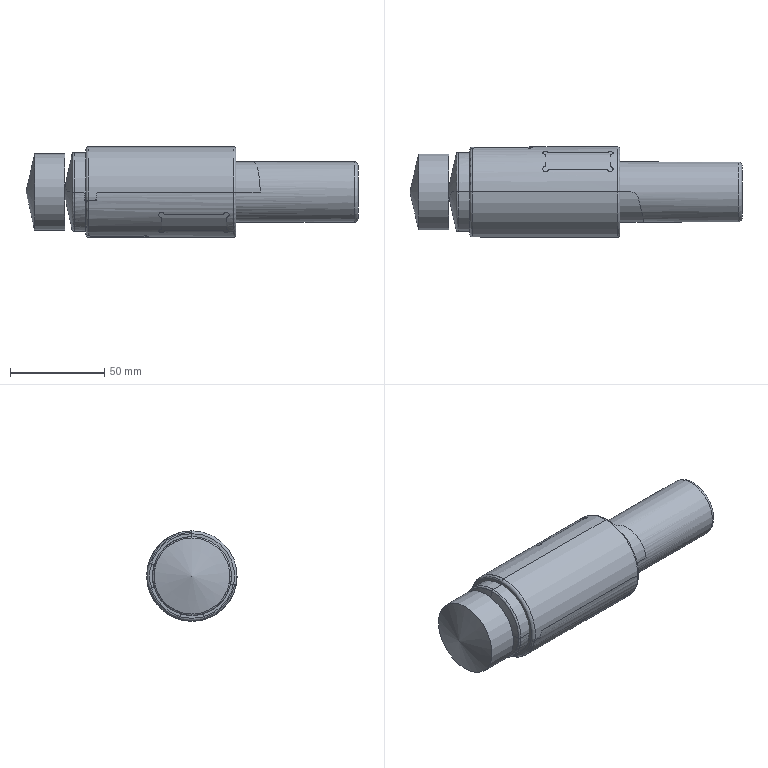NC program | NX | posted with a generic post | part box 176.413 x 48 x 48 mm
Lines 1742 to 2818 of 71815:
(ZLEVEL_PROFILE_COPY , TOOL : D10)
N3482 T10 M6
N3484 G54
N3486 G17 G0 G90 X-59.96 Y-8.562 S3500 M3
N3488 G43 Z33.936 H10
N3490 Z15.781
N3492 G94 G1 X-59.542 Y-8.165 F2000.
N3494 G3 X-59.258 Y-7.206 R1.
N3496 G1 X-59.789 Y-5.
N3498 X-62.069
N3500 G3 X-62.935 Y-5.5 R1.
N3502 G1 X-63.224 Y-6.
N3504 G0 X-59.96 Y-8.563 Z15.562
N3506 G1 X-59.541 Y-8.165
N3508 G3 X-59.258 Y-7.206 R1.
N3510 G1 X-59.789 Y-5.
N3512 X-62.069
N3514 G3 X-62.935 Y-5.5 R1.
N3516 G1 X-63.224 Y-6.
N3518 G0 X-59.96 Y-8.563 Z15.342
N3520 G1 X-59.541 Y-8.166
N3522 G3 X-59.258 Y-7.207 R1.
N3524 G1 X-59.789 Y-5.
N3526 X-62.07
N3528 G3 X-62.936 Y-5.5 R1.
N3530 G1 X-63.224 Y-6.
N3532 G0 X-59.96 Y-8.564 Z15.123
N3534 G1 X-59.541 Y-8.166
N3536 G3 X-59.258 Y-7.207 R1.
N3538 G1 X-59.789 Y-5.
N3540 X-62.07
N3542 G3 X-62.936 Y-5.5 R1.
N3544 G1 X-63.225 Y-6.
N3546 G0 X-59.96 Y-8.565 Z14.904
N3548 G1 X-59.541 Y-8.167
N3550 G3 X-59.257 Y-7.208 R1.
N3552 G1 X-59.789 Y-5.
N3554 X-62.07
N3556 G3 X-62.936 Y-5.5 R1.
N3558 G1 X-63.225 Y-6.
N3560 G0 X-59.959 Y-8.569 Z14.685
N3562 G1 X-59.54 Y-8.171
N3564 G3 X-59.256 Y-7.212 R1.
N3566 G1 X-59.789 Y-5.
N3568 X-62.071
N3570 G3 X-62.937 Y-5.5 R1.
N3572 G1 X-63.225 Y-6.
N3574 G0 X-59.959 Y-8.569 Z14.466
N3576 G1 X-59.54 Y-8.171
N3578 G3 X-59.256 Y-7.212 R1.
N3580 G1 X-59.789 Y-5.
N3582 X-62.071
N3584 G3 X-62.937 Y-5.5 R1.
N3586 G1 X-63.226 Y-6.
N3588 G0 X-59.959 Y-8.569 Z14.247
N3590 G1 X-59.54 Y-8.171
N3592 G3 X-59.256 Y-7.212 R1.
N3594 G1 X-59.789 Y-5.
N3596 X-62.071
N3598 G3 X-62.937 Y-5.5 R1.
N3600 G1 X-63.226 Y-6.
N3602 G0 X-59.959 Y-8.569 Z14.027
N3604 G1 X-59.54 Y-8.171
N3606 G3 X-59.256 Y-7.212 R1.
N3608 G1 X-59.789 Y-5.
N3610 X-62.072
N3612 G3 X-62.938 Y-5.5 R1.
N3614 G1 X-63.226 Y-6.
N3616 G0 X-59.959 Y-8.569 Z13.808
N3618 G1 X-59.54 Y-8.171
N3620 G3 X-59.256 Y-7.212 R1.
N3622 G1 X-59.789 Y-5.
N3624 X-62.072
N3626 G3 X-62.938 Y-5.5 R1.
N3628 G1 X-63.227 Y-6.
N3630 G0 X-59.959 Y-8.569 Z13.589
N3632 G1 X-59.54 Y-8.171
N3634 G3 X-59.256 Y-7.212 R1.
N3636 G1 X-59.789 Y-5.
N3638 X-62.072
N3640 G3 X-62.939 Y-5.5 R1.
N3642 G1 X-63.227 Y-6.
N3644 G0 X-59.959 Y-8.569 Z13.37
N3646 G1 X-59.54 Y-8.171
N3648 G3 X-59.256 Y-7.212 R1.
N3650 G1 X-59.789 Y-5.
N3652 X-62.073
N3654 G3 X-62.939 Y-5.5 R1.
N3656 G1 X-63.228 Y-6.
N3658 G0 X-59.959 Y-8.569 Z13.151
N3660 G1 X-59.54 Y-8.171
N3662 G3 X-59.256 Y-7.212 R1.
N3664 G1 X-59.789 Y-5.
N3666 X-62.073
N3668 G3 X-62.939 Y-5.5 R1.
N3670 G1 X-63.228 Y-6.
N3672 G0 X-59.959 Y-8.569 Z12.932
N3674 G1 X-59.54 Y-8.171
N3676 G3 X-59.256 Y-7.212 R1.
N3678 G1 X-59.789 Y-5.
N3680 X-62.073
N3682 G3 X-62.939 Y-5.5 R1.
N3684 G1 X-63.228 Y-6.
N3686 G0 X-59.959 Y-8.569 Z12.712
N3688 G1 X-59.54 Y-8.171
N3690 G3 X-59.256 Y-7.212 R1.
N3692 G1 X-59.789 Y-5.
N3694 X-62.073
N3696 G3 X-62.939 Y-5.5 R1.
N3698 G1 X-63.228 Y-6.
N3700 G0 X-59.959 Y-8.569 Z12.493
N3702 G1 X-59.54 Y-8.171
N3704 G3 X-59.256 Y-7.212 R1.
N3706 G1 X-59.789 Y-5.
N3708 X-62.073
N3710 G3 X-62.939 Y-5.5 R1.
N3712 G1 X-63.228 Y-6.
N3714 G0 X-59.959 Y-8.569 Z12.274
N3716 G1 X-59.54 Y-8.171
N3718 G3 X-59.256 Y-7.212 R1.
N3720 G1 X-59.789 Y-5.
N3722 X-62.073
N3724 G3 X-62.939 Y-5.5 R1.
N3726 G1 X-63.228 Y-6.
N3728 G0 X-59.959 Y-8.569 Z12.055
N3730 G1 X-59.54 Y-8.171
N3732 G3 X-59.256 Y-7.212 R1.
N3734 G1 X-59.789 Y-5.
N3736 X-62.074
N3738 G3 X-62.94 Y-5.5 R1.
N3740 G1 X-63.228 Y-6.
N3742 G0 X-59.962 Y-8.556 Z11.836
N3744 G1 X-59.543 Y-8.158
N3746 G3 X-59.26 Y-7.199 R1.
N3748 G1 X-59.788 Y-5.001
N3750 X-62.049
N3752 G3 X-62.915 Y-5.501 R1.
N3754 G1 X-63.204 Y-6.001
N3756 G0 X-59.961 Y-8.561 Z11.616
N3758 G1 X-59.542 Y-8.163
N3760 G3 X-59.258 Y-7.204 R1.
N3762 G1 X-59.787 Y-5.006
N3764 X-62.048
N3766 G3 X-62.914 Y-5.506 R1.
N3768 G1 X-63.203 Y-6.006
N3770 G0 X-59.958 Y-8.57 Z11.397
N3772 G1 X-59.54 Y-8.172
N3774 G3 X-59.256 Y-7.213 R1.
N3776 G1 X-59.785 Y-5.015
N3778 X-62.046
N3780 G3 X-62.912 Y-5.515 R1.
N3782 G1 X-63.201 Y-6.015
N3784 G0 X-59.955 Y-8.583 Z11.178
N3786 G1 X-59.537 Y-8.185
N3788 G3 X-59.253 Y-7.226 R1.
N3790 G1 X-59.782 Y-5.028
N3792 X-62.043
N3794 G3 X-62.909 Y-5.528 R1.
N3796 G1 X-63.197 Y-6.028
N3798 G0 X-59.951 Y-8.6 Z10.959
N3800 G1 X-59.532 Y-8.202
N3802 G3 X-59.249 Y-7.244 R1.
N3804 G1 X-59.778 Y-5.045
N3806 X-62.039
N3808 G3 X-62.905 Y-5.545 R1.
N3810 G1 X-63.193 Y-6.045
N3812 G0 X-59.946 Y-8.621 Z10.74
N3814 G1 X-59.527 Y-8.224
N3816 G3 X-59.244 Y-7.265 R1.
N3818 G1 X-59.773 Y-5.066
N3820 X-62.034
N3822 G3 X-62.9 Y-5.566 R1.
N3824 G1 X-63.188 Y-6.066
N3826 G0 X-59.94 Y-8.646 Z10.521
N3828 G1 X-59.521 Y-8.249
N3830 G3 X-59.238 Y-7.29 R1.
N3832 G1 X-59.767 Y-5.092
N3834 X-62.027
N3836 G3 X-62.894 Y-5.592 R1.
N3838 G1 X-63.182 Y-6.092
N3840 G0 X-59.933 Y-8.676 Z10.301
N3842 G1 X-59.514 Y-8.278
N3844 G3 X-59.231 Y-7.319 R1.
N3846 G1 X-59.759 Y-5.121
N3848 X-62.02
N3850 G3 X-62.886 Y-5.621 R1.
N3852 G1 X-63.175 Y-6.121
N3854 G0 X-59.925 Y-8.709 Z10.082
N3856 G1 X-59.506 Y-8.311
N3858 G3 X-59.223 Y-7.352 R1.
N3860 G1 X-59.751 Y-5.154
N3862 X-62.012
N3864 G3 X-62.878 Y-5.654 R1.
N3866 G1 X-63.167 Y-6.154
N3868 G0 X-59.916 Y-8.747 Z9.863
N3870 G1 X-59.497 Y-8.349
N3872 G3 X-59.214 Y-7.39 R1.
N3874 G1 X-59.742 Y-5.192
N3876 X-62.003
N3878 G3 X-62.869 Y-5.692 R1.
N3880 G1 X-63.158 Y-6.192
N3882 G0 X-59.906 Y-8.788 Z9.644
N3884 G1 X-59.487 Y-8.391
N3886 G3 X-59.204 Y-7.432 R1.
N3888 G1 X-59.732 Y-5.234
N3890 X-61.993
N3892 G3 X-62.859 Y-5.734 R1.
N3894 G1 X-63.148 Y-6.234
N3896 G0 X-59.895 Y-8.834 Z9.425
N3898 G1 X-59.476 Y-8.437
N3900 G3 X-59.193 Y-7.478 R1.
N3902 G1 X-59.721 Y-5.28
N3904 X-61.982
N3906 G3 X-62.848 Y-5.78 R1.
N3908 G1 X-63.137 Y-6.28
N3910 G0 X-59.883 Y-8.885 Z9.205
N3912 G1 X-59.464 Y-8.487
N3914 G3 X-59.18 Y-7.528 R1.
N3916 G1 X-59.709 Y-5.33
N3918 X-61.97
N3920 G3 X-62.836 Y-5.83 R1.
N3922 G1 X-63.125 Y-6.33
N3924 G0 X-59.869 Y-8.939 Z8.986
N3926 G1 X-59.451 Y-8.542
N3928 G3 X-59.167 Y-7.583 R1.
N3930 G1 X-59.696 Y-5.385
N3932 X-61.957
N3934 G3 X-62.823 Y-5.885 R1.
N3936 G1 X-63.112 Y-6.385
N3938 G0 X-59.855 Y-8.998 Z8.767
N3940 G1 X-59.437 Y-8.601
N3942 G3 X-59.153 Y-7.642 R1.
N3944 G1 X-59.682 Y-5.444
N3946 X-61.943
N3948 G3 X-62.809 Y-5.944 R1.
N3950 G1 X-63.097 Y-6.444
N3952 G0 X-59.84 Y-9.062 Z8.548
N3954 G1 X-59.421 Y-8.664
N3956 G3 X-59.138 Y-7.706 R1.
N3958 G1 X-59.667 Y-5.507
N3960 X-61.927
N3962 G3 X-62.794 Y-6.007 R1.
N3964 G1 X-63.082 Y-6.507
N3966 G0 X-59.824 Y-9.13 Z8.329
N3968 G1 X-59.405 Y-8.733
N3970 G3 X-59.121 Y-7.774 R1.
N3972 G1 X-59.65 Y-5.575
N3974 X-61.911
N3976 G3 X-62.777 Y-6.075 R1.
N3978 G1 X-63.066 Y-6.575
N3980 G0 X-59.806 Y-9.203 Z8.11
N3982 G1 X-59.387 Y-8.805
N3984 G3 X-59.104 Y-7.846 R1.
N3986 G1 X-59.633 Y-5.648
N3988 X-61.894
N3990 G3 X-62.76 Y-6.148 R1.
N3992 G1 X-63.048 Y-6.648
N3994 G0 X-59.787 Y-9.28 Z7.89
N3996 G1 X-59.369 Y-8.883
N3998 G3 X-59.085 Y-7.924 R1.
N4000 G1 X-59.614 Y-5.726
N4002 X-61.875
N4004 G3 X-62.741 Y-6.226 R1.
N4006 G1 X-63.03 Y-6.726
N4008 G0 X-59.768 Y-9.363 Z7.671
N4010 G1 X-59.349 Y-8.965
N4012 G3 X-59.065 Y-8.006 R1.
N4014 G1 X-59.594 Y-5.808
N4016 X-61.855
N4018 G3 X-62.721 Y-6.308 R1.
N4020 G1 X-63.01 Y-6.808
N4022 G0 X-59.747 Y-9.45 Z7.452
N4024 G1 X-59.328 Y-9.052
N4026 G3 X-59.044 Y-8.093 R1.
N4028 G1 X-59.573 Y-5.895
N4030 X-61.834
N4032 G3 X-62.7 Y-6.395 R1.
N4034 G1 X-62.989 Y-6.895
N4036 G0 X-59.724 Y-9.542 Z7.233
N4038 G1 X-59.306 Y-9.145
N4040 G3 X-59.022 Y-8.186 R1.
N4042 G1 X-59.551 Y-5.988
N4044 X-61.812
N4046 G3 X-62.678 Y-6.488 R1.
N4048 G1 X-62.967 Y-6.988
N4050 G0 X-59.701 Y-9.64 Z7.014
N4052 G1 X-59.282 Y-9.242
N4054 G3 X-58.999 Y-8.283 R1.
N4056 G1 X-59.528 Y-6.085
N4058 X-61.789
N4060 G3 X-62.655 Y-6.585 R1.
N4062 G1 X-62.943 Y-7.085
N4064 G0 X-59.676 Y-9.743 Z6.795
N4066 G1 X-59.258 Y-9.345
N4068 G3 X-58.974 Y-8.386 R1.
N4070 G1 X-59.503 Y-6.188
N4072 X-61.764
N4074 G3 X-62.63 Y-6.688 R1.
N4076 G1 X-62.918 Y-7.188
N4078 G0 X-59.65 Y-9.851 Z6.575
N4080 G1 X-59.232 Y-9.453
N4082 G3 X-58.948 Y-8.494 R1.
N4084 G1 X-59.477 Y-6.296
N4086 X-61.738
N4088 G3 X-62.604 Y-6.796 R1.
N4090 G1 X-62.892 Y-7.296
N4092 G0 X-59.623 Y-9.965 Z6.356
N4094 G1 X-59.204 Y-9.567
N4096 G3 X-58.921 Y-8.608 R1.
N4098 G1 X-59.449 Y-6.41
N4100 X-61.71
N4102 G3 X-62.576 Y-6.91 R1.
N4104 G1 X-62.865 Y-7.41
N4106 G0 X-59.594 Y-10.085 Z6.137
N4108 G1 X-59.175 Y-9.687
N4110 G3 X-58.892 Y-8.728 R1.
N4112 G1 X-59.421 Y-6.53
N4114 X-61.682
N4116 G3 X-62.548 Y-7.03 R1.
N4118 G1 X-62.836 Y-7.53
N4120 G0 X-59.564 Y-10.21 Z5.918
N4122 G1 X-59.145 Y-9.813
N4124 G3 X-58.862 Y-8.854 R1.
N4126 G1 X-59.39 Y-6.656
N4128 X-61.651
N4130 G3 X-62.517 Y-7.156 R1.
N4132 G1 X-62.806 Y-7.656
N4134 G0 X-59.532 Y-10.342 Z5.699
N4136 G1 X-59.113 Y-9.945
N4138 G3 X-58.83 Y-8.986 R1.
N4140 G1 X-59.359 Y-6.788
N4142 X-61.62
N4144 G3 X-62.486 Y-7.288 R1.
N4146 G1 X-62.774 Y-7.788
N4148 G0 X-59.499 Y-10.481 Z5.479
N4150 G1 X-59.08 Y-10.083
N4152 G3 X-58.796 Y-9.124 R1.
N4154 G1 X-59.325 Y-6.926
N4156 X-61.586
N4158 G3 X-62.452 Y-7.426 R1.
N4160 G1 X-62.741 Y-7.926
N4162 G0 X-59.464 Y-10.626 Z5.26
N4164 G1 X-59.045 Y-10.229
N4166 G3 X-58.762 Y-9.27 R1.
N4168 G1 X-59.29 Y-7.071
N4170 X-61.551
N4172 G3 X-62.417 Y-7.571 R1.
N4174 G1 X-62.706 Y-8.071
N4176 G0 X-59.427 Y-10.779 Z5.041
N4178 G1 X-59.008 Y-10.381
N4180 G3 X-58.725 Y-9.422 R1.
N4182 G1 X-59.254 Y-7.224
N4184 X-61.515
N4186 G3 X-62.381 Y-7.724 R1.
N4188 G1 X-62.669 Y-8.224
N4190 G0 X-59.389 Y-10.938 Z4.822
N4192 G1 X-58.97 Y-10.541
N4194 G3 X-58.686 Y-9.582 R1.
N4196 G1 X-59.215 Y-7.384
N4198 X-61.476
N4200 G3 X-62.342 Y-7.884 R1.
N4202 G1 X-62.631 Y-8.384
N4204 G0 X-59.348 Y-11.106 Z4.603
N4206 G1 X-58.93 Y-10.708
N4208 G3 X-58.646 Y-9.749 R1.
N4210 G1 X-59.175 Y-7.551
N4212 X-61.436
N4214 G3 X-62.302 Y-8.051 R1.
N4216 G1 X-62.591 Y-8.551
N4218 G0 X-59.306 Y-11.282 Z4.384
N4220 G1 X-58.887 Y-10.884
N4222 G3 X-58.604 Y-9.925 R1.
N4224 G1 X-59.133 Y-7.727
N4226 X-61.394
N4228 G3 X-62.26 Y-8.227 R1.
N4230 G1 X-62.548 Y-8.727
N4232 G0 X-59.262 Y-11.466 Z4.164
N4234 G1 X-58.843 Y-11.069
N4236 G3 X-58.559 Y-10.11 R1.
N4238 G1 X-59.088 Y-7.911
N4240 X-61.349
N4242 G3 X-62.215 Y-8.411 R1.
N4244 G1 X-62.504 Y-8.911
N4246 G0 X-59.215 Y-11.66 Z3.945
N4248 G1 X-58.796 Y-11.262
N4250 G3 X-58.513 Y-10.303 R1.
N4252 G1 X-59.042 Y-8.105
N4254 X-61.303
N4256 G3 X-62.169 Y-8.605 R1.
N4258 G1 X-62.457 Y-9.105
N4260 G0 X-59.166 Y-11.863 Z3.726
N4262 G1 X-58.748 Y-11.466
N4264 G3 X-58.464 Y-10.507 R1.
N4266 G1 X-58.993 Y-8.309
N4268 X-61.254
N4270 G3 X-62.12 Y-8.809 R1.
N4272 G1 X-62.408 Y-9.309
N4274 G0 X-59.115 Y-12.077 Z3.507
N4276 G1 X-58.696 Y-11.68
N4278 G3 X-58.412 Y-10.721 R1.
N4280 G1 X-58.941 Y-8.523
N4282 X-61.202
N4284 G3 X-62.068 Y-9.023 R1.
N4286 G1 X-62.357 Y-9.523
N4288 G0 X-59.06 Y-12.303 Z3.288
N4290 G1 X-58.642 Y-11.905
N4292 G3 X-58.358 Y-10.946 R1.
N4294 G1 X-58.887 Y-8.748
N4296 X-61.148
N4298 G3 X-62.014 Y-9.248 R1.
N4300 G1 X-62.303 Y-9.748
N4302 G0 X-59.003 Y-12.541 Z3.068
N4304 G1 X-58.585 Y-12.143
N4306 G3 X-58.301 Y-11.184 R1.
N4308 G1 X-58.83 Y-8.986
N4310 X-61.091
N4312 G3 X-61.957 Y-9.486 R1.
N4314 G1 X-62.245 Y-9.986
N4316 G0 X-58.943 Y-12.792 Z2.849
N4318 G1 X-58.524 Y-12.394
N4320 G3 X-58.241 Y-11.435 R1.
N4322 G1 X-58.769 Y-9.237
N4324 X-61.03
N4326 G3 X-61.896 Y-9.737 R1.
N4328 G1 X-62.185 Y-10.237
N4330 G0 X-58.879 Y-13.058 Z2.63
N4332 G1 X-58.46 Y-12.66
N4334 G3 X-58.177 Y-11.701 R1.
N4336 G1 X-58.705 Y-9.503
N4338 X-60.966
N4340 G3 X-61.832 Y-10.003 R1.
N4342 G1 X-62.121 Y-10.503
N4344 G0 X-58.811 Y-13.34 Z2.411
N4346 G1 X-58.392 Y-12.943
N4348 G3 X-58.109 Y-11.984 R1.
N4350 G1 X-58.637 Y-9.785
N4352 X-60.898
N4354 G3 X-61.764 Y-10.285 R1.
N4356 G1 X-62.053 Y-10.785
N4358 G0 X-58.739 Y-13.641 Z2.192
N4360 G1 X-58.32 Y-13.244
N4362 G3 X-58.036 Y-12.285 R1.
N4364 G1 X-58.565 Y-10.086
N4366 X-60.826
N4368 G3 X-61.692 Y-10.586 R1.
N4370 G1 X-61.981 Y-11.086
N4372 G0 X-58.661 Y-13.963 Z1.973
N4374 G1 X-58.242 Y-13.565
N4376 G3 X-57.959 Y-12.606 R1.
N4378 G1 X-58.488 Y-10.408
N4380 X-60.749
N4382 G3 X-61.615 Y-10.908 R1.
N4384 G1 X-61.903 Y-11.408
N4386 G0 X-58.578 Y-14.309 Z1.753
N4388 G1 X-58.159 Y-13.912
N4390 G3 X-57.876 Y-12.953 R1.
N4392 G1 X-58.404 Y-10.754
N4394 X-60.665
N4396 G3 X-61.531 Y-11.254 R1.
N4398 G1 X-61.82 Y-11.754
N4400 G0 X-58.488 Y-14.684 Z1.534
N4402 G1 X-58.069 Y-14.286
N4404 G3 X-57.786 Y-13.327 R1.
N4406 G1 X-58.314 Y-11.129
N4408 X-60.575
N4410 G3 X-61.441 Y-11.629 R1.
N4412 G1 X-61.73 Y-12.129
N4414 G0 X-58.389 Y-15.093 Z1.315
N4416 G1 X-57.971 Y-14.695
N4418 G3 X-57.687 Y-13.736 R1.
N4420 G1 X-58.216 Y-11.538
N4422 X-60.477
N4424 G3 X-61.343 Y-12.038 R1.
N4426 G1 X-61.632 Y-12.538
N4428 G0 X-58.281 Y-15.545 Z1.096
N4430 G1 X-57.862 Y-15.147
N4432 G3 X-57.578 Y-14.188 R1.
N4434 G1 X-58.107 Y-11.99
N4436 X-60.368
N4438 G3 X-61.234 Y-12.49 R1.
N4440 G1 X-61.523 Y-12.99
N4442 G0 X-58.159 Y-16.052 Z0.877
N4444 G1 X-57.74 Y-15.655
N4446 G3 X-57.456 Y-14.696 R1.
N4448 G1 X-57.985 Y-12.498
N4450 X-60.246
N4452 G3 X-61.112 Y-12.998 R1.
N4454 G1 X-61.401 Y-13.498
N4456 G0 X-58.018 Y-16.637 Z0.658
N4458 G1 X-57.599 Y-16.239
N4460 G3 X-57.316 Y-15.281 R1.
N4462 G1 X-57.844 Y-13.082
N4464 X-60.105
N4466 G3 X-60.971 Y-13.582 R1.
N4468 G1 X-61.26 Y-14.082
N4470 G0 X-57.842 Y-17.368 Z0.438
N4472 G1 X-57.424 Y-16.97
N4474 G3 X-57.14 Y-16.011 R1.
N4476 G1 X-57.675 Y-13.786
N4478 X-59.942
N4480 G3 X-60.808 Y-14.286 R1.
N4482 G1 X-61.097 Y-14.786
N4484 G0 X-57.613 Y-18.321 Z0.219
N4486 G1 X-57.194 Y-17.923
N4488 G3 X-56.911 Y-16.964 R1.
N4490 G1 X-57.451 Y-14.717
N4492 X-59.723
N4494 G3 X-60.589 Y-15.217 R1.
N4496 G1 X-60.877 Y-15.717
N4498 G0 X-57.177 Y-20.13 Z0.
N4500 G1 X-56.758 Y-19.732
N4502 G3 X-56.475 Y-18.773 R1.
N4504 G1 X-56.814 Y-17.369
N4506 X-56.861 Y-17.169
N4508 X-57.007 Y-16.563
N4510 X-59.331
N4512 G3 X-60.197 Y-17.064 R1.
N4514 G1 X-60.486 Y-17.564
N4516 G0 Z30.274
(ZLEVEL_PROFILE_COPY_COPY , TOOL : D10)
N4518 X-80.529 Y25.398 S2500
N4520 Z24.082
N4522 Y18.689 Z17.374
N4524 G1 X-99.3 Y17.993 Z16.678 F1000.
N4526 Y16.609 Z17.924
N4528 X-87.2 Y16.161 Z17.476
N4530 X-75.1 F2000.
N4532 Y17.476 Z16.161
N4534 X-99.3
N4536 Y16.161 Z17.476
N4538 X-87.2
N4540 X-75.15 Y16.012 Z17.327
N4542 X-75.1 Y16.043 Z17.293
N4544 Y16.177 Z17.154
N4546 Y17.323 Z16.008
N4548 X-99.3
N4550 Y16.008 Z17.323
N4552 X-87.2
N4554 X-75.15 Y15.86 Z17.175
N4556 X-75.1 Y15.891 Z17.141
N4558 Y16.025 Z17.002
N4560 Y17.171 Z15.856
N4562 X-99.3
N4564 Y15.856 Z17.171
N4566 X-87.2
N4568 X-75.15 Y15.707 Z17.022
N4570 X-75.1 Y15.739 Z16.989
N4572 Y15.873 Z16.85
N4574 Y17.019 Z15.704
N4576 X-99.3
N4578 Y15.704 Z17.019
N4580 X-87.2
N4582 X-75.15 Y15.555 Z16.87
N4584 X-75.1 Y15.586 Z16.836
N4586 Y15.72 Z16.698
N4588 Y16.867 Z15.551
N4590 X-99.3
N4592 Y15.551 Z16.867
N4594 X-87.2
N4596 X-75.15 Y15.403 Z16.718
N4598 X-75.1 Y15.434 Z16.684
N4600 Y15.568 Z16.545
N4602 Y16.714 Z15.399
N4604 X-99.3
N4606 Y15.399 Z16.714
N4608 X-87.2
N4610 X-75.15 Y15.25 Z16.566
N4612 X-75.1 Y15.282 Z16.532
N4614 Y15.416 Z16.393
N4616 Y16.562 Z15.247
N4618 X-99.3
N4620 Y15.247 Z16.562
N4622 X-87.2
N4624 X-75.15 Y15.098 Z16.413
N4626 X-75.1 Y15.13 Z16.379
N4628 Y15.263 Z16.241
N4630 Y16.41 Z15.094
N4632 X-99.3
N4634 Y15.094 Z16.41
N4636 X-87.2
N4638 X-75.15 Y14.946 Z16.261
N4640 X-75.1 Y14.977 Z16.227
N4642 Y15.111 Z16.088
N4644 Y16.257 Z14.942
N4646 X-99.3
N4648 Y14.942 Z16.257
N4650 X-87.2
N4652 X-75.15 Y14.793 Z16.109
N4654 X-75.1 Y14.825 Z16.075
N4656 Y14.959 Z15.936
N4658 Y16.105 Z14.79
N4660 X-99.3
N4662 Y14.79 Z16.105
N4664 X-87.2
N4666 X-75.15 Y14.641 Z15.956
N4668 X-75.1 Y14.673 Z15.923
N4670 Y14.807 Z15.784
N4672 Y15.953 Z14.638
N4674 X-99.3
N4676 Y14.638 Z15.953
N4678 X-87.2
N4680 X-75.15 Y14.489 Z15.804
N4682 X-75.1 Y14.52 Z15.77
N4684 Y14.654 Z15.631
N4686 Y15.801 Z14.485
N4688 X-99.3
N4690 Y14.485 Z15.801
N4692 X-87.2
N4694 X-75.15 Y14.337 Z15.652
N4696 X-75.1 Y14.368 Z15.618
N4698 Y14.502 Z15.479
N4700 Y15.648 Z14.333
N4702 X-99.3
N4704 Y14.333 Z15.648
N4706 X-87.2
N4708 X-75.15 Y14.184 Z15.499
N4710 X-75.1 Y14.216 Z15.466
N4712 Y14.35 Z15.327
N4714 Y15.496 Z14.181
N4716 X-99.3
N4718 Y14.181 Z15.496
N4720 X-87.2
N4722 X-75.15 Y14.032 Z15.347
N4724 X-75.1 Y14.063 Z15.313
N4726 Y14.197 Z15.175
N4728 Y15.344 Z14.028
N4730 X-99.3
N4732 Y14.028 Z15.344
N4734 X-87.2
N4736 X-75.15 Y13.88 Z15.195
N4738 X-75.1 Y13.911 Z15.161
N4740 Y14.045 Z15.022
N4742 Y15.191 Z13.876
N4744 X-99.3
N4746 Y13.876 Z15.191
N4748 X-87.2
N4750 X-75.15 Y13.727 Z15.043
N4752 X-75.1 Y13.759 Z15.009
N4754 Y13.893 Z14.87
N4756 Y15.039 Z13.724
N4758 X-99.3
N4760 Y13.724 Z15.039
N4762 X-87.2
N4764 X-75.15 Y13.575 Z14.89
N4766 X-75.1 Y13.607 Z14.856
N4768 Y13.741 Z14.718
N4770 Y14.887 Z13.572
N4772 X-99.3
N4774 Y13.572 Z14.887
N4776 X-87.2
N4778 X-75.15 Y13.423 Z14.738
N4780 X-75.1 Y13.454 Z14.704
N4782 Y13.588 Z14.565
N4784 Y14.734 Z13.419
N4786 X-99.3
N4788 Y13.419 Z14.734
N4790 X-87.2
N4792 X-75.15 Y13.27 Z14.586
N4794 X-75.1 Y13.302 Z14.552
N4796 Y13.436 Z14.413
N4798 Y14.582 Z13.267
N4800 X-99.3
N4802 Y13.267 Z14.582
N4804 X-87.2
N4806 X-75.15 Y13.118 Z14.433
N4808 X-75.1 Y13.15 Z14.4
N4810 Y13.284 Z14.261
N4812 Y14.43 Z13.115
N4814 X-99.3
N4816 Y13.115 Z14.43
N4818 X-87.2
N4820 X-75.15 Y12.966 Z14.281
N4822 X-75.1 Y12.997 Z14.247
N4824 Y13.131 Z14.109
N4826 Y14.278 Z12.962
N4828 X-99.3
N4830 Y12.962 Z14.278
N4832 X-87.2
N4834 X-75.15 Y12.814 Z14.129
N4836 X-75.1 Y12.845 Z14.095
N4838 Y12.979 Z13.956
N4840 Y14.125 Z12.81
N4842 X-99.3
N4844 Y12.81 Z14.125
N4846 X-87.2
N4848 X-75.15 Y12.661 Z13.977
N4850 X-75.1 Y12.693 Z13.943
N4852 Y12.827 Z13.804
N4854 Y13.973 Z12.658
N4856 X-99.3
N4858 Y12.658 Z13.973
N4860 X-87.2
N4862 X-75.15 Y12.509 Z13.824
N4864 X-75.1 Y12.541 Z13.79
N4866 Y12.674 Z13.652
N4868 Y13.821 Z12.505
N4870 X-99.3
N4872 Y12.505 Z13.821
N4874 X-75.1
N4876 Y12.674 Z13.652
N4878 Y13.735 Z14.712
N4880 G0 Y24.255 Z25.233
(ZLEVEL_PROFILE_COPY_COPY_COPY_1 , TOOL : D10)
N4882 X-80.529 Y-25.398
N4884 Z-24.082
N4886 Y-18.689 Z-17.374
N4888 G1 X-99.3 Y-17.993 Z-16.678 F1000.
N4890 Y-16.609 Z-17.924
N4892 X-87.2 Y-16.161 Z-17.476
N4894 X-75.1 F2000.
N4896 Y-17.476 Z-16.161
N4898 X-99.3
N4900 Y-16.161 Z-17.476
N4902 X-87.2
N4904 X-75.15 Y-16.012 Z-17.327
N4906 X-75.1 Y-16.043 Z-17.293
N4908 Y-16.177 Z-17.154
N4910 Y-17.323 Z-16.008
N4912 X-99.3
N4914 Y-16.008 Z-17.323
N4916 X-87.2
N4918 X-75.15 Y-15.86 Z-17.175
N4920 X-75.1 Y-15.891 Z-17.141
N4922 Y-16.025 Z-17.002
N4924 Y-17.171 Z-15.856
N4926 X-99.3
N4928 Y-15.856 Z-17.171
N4930 X-87.2
N4932 X-75.15 Y-15.707 Z-17.022
N4934 X-75.1 Y-15.739 Z-16.989
N4936 Y-15.873 Z-16.85
N4938 Y-17.019 Z-15.704
N4940 X-99.3
N4942 Y-15.704 Z-17.019
N4944 X-87.2
N4946 X-75.15 Y-15.555 Z-16.87
N4948 X-75.1 Y-15.586 Z-16.836
N4950 Y-15.72 Z-16.698
N4952 Y-16.867 Z-15.551
N4954 X-99.3
N4956 Y-15.551 Z-16.867
N4958 X-87.2
N4960 X-75.15 Y-15.403 Z-16.718
N4962 X-75.1 Y-15.434 Z-16.684
N4964 Y-15.568 Z-16.545
N4966 Y-16.714 Z-15.399
N4968 X-99.3
N4970 Y-15.399 Z-16.714
N4972 X-87.2
N4974 X-75.15 Y-15.25 Z-16.566
N4976 X-75.1 Y-15.282 Z-16.532
N4978 Y-15.416 Z-16.393
N4980 Y-16.562 Z-15.247
N4982 X-99.3
N4984 Y-15.247 Z-16.562
N4986 X-87.2
N4988 X-75.15 Y-15.098 Z-16.413
N4990 X-75.1 Y-15.13 Z-16.379
N4992 Y-15.263 Z-16.241
N4994 Y-16.41 Z-15.094
N4996 X-99.3
N4998 Y-15.094 Z-16.41
N5000 X-87.2
N5002 X-75.15 Y-14.946 Z-16.261
N5004 X-75.1 Y-14.977 Z-16.227
N5006 Y-15.111 Z-16.088
N5008 Y-16.257 Z-14.942
N5010 X-99.3
N5012 Y-14.942 Z-16.257
N5014 X-87.2
N5016 X-75.15 Y-14.793 Z-16.109
N5018 X-75.1 Y-14.825 Z-16.075
N5020 Y-14.959 Z-15.936
N5022 Y-16.105 Z-14.79
N5024 X-99.3
N5026 Y-14.79 Z-16.105
N5028 X-87.2
N5030 X-75.15 Y-14.641 Z-15.956
N5032 X-75.1 Y-14.673 Z-15.923
N5034 Y-14.807 Z-15.784
N5036 Y-15.953 Z-14.638
N5038 X-99.3
N5040 Y-14.638 Z-15.953
N5042 X-87.2
N5044 X-75.15 Y-14.489 Z-15.804
N5046 X-75.1 Y-14.52 Z-15.77
N5048 Y-14.654 Z-15.631
N5050 Y-15.801 Z-14.485
N5052 X-99.3
N5054 Y-14.485 Z-15.801
N5056 X-87.2
N5058 X-75.15 Y-14.337 Z-15.652
N5060 X-75.1 Y-14.368 Z-15.618
N5062 Y-14.502 Z-15.479
N5064 Y-15.648 Z-14.333
N5066 X-99.3
N5068 Y-14.333 Z-15.648
N5070 X-87.2
N5072 X-75.15 Y-14.184 Z-15.499
N5074 X-75.1 Y-14.216 Z-15.466
N5076 Y-14.35 Z-15.327
N5078 Y-15.496 Z-14.181
N5080 X-99.3
N5082 Y-14.181 Z-15.496
N5084 X-87.2
N5086 X-75.15 Y-14.032 Z-15.347
N5088 X-75.1 Y-14.063 Z-15.313
N5090 Y-14.197 Z-15.175
N5092 Y-15.344 Z-14.028
N5094 X-99.3
N5096 Y-14.028 Z-15.344
N5098 X-87.2
N5100 X-75.15 Y-13.88 Z-15.195
N5102 X-75.1 Y-13.911 Z-15.161
N5104 Y-14.045 Z-15.022
N5106 Y-15.191 Z-13.876
N5108 X-99.3
N5110 Y-13.876 Z-15.191
N5112 X-87.2
N5114 X-75.15 Y-13.727 Z-15.043
N5116 X-75.1 Y-13.759 Z-15.009
N5118 Y-13.893 Z-14.87
N5120 Y-15.039 Z-13.724
N5122 X-99.3
N5124 Y-13.724 Z-15.039
N5126 X-87.2
N5128 X-75.15 Y-13.575 Z-14.89
N5130 X-75.1 Y-13.607 Z-14.856
N5132 Y-13.741 Z-14.718
N5134 Y-14.887 Z-13.572
N5136 X-99.3
N5138 Y-13.572 Z-14.887
N5140 X-87.2
N5142 X-75.15 Y-13.423 Z-14.738
N5144 X-75.1 Y-13.454 Z-14.704
N5146 Y-13.588 Z-14.565
N5148 Y-14.734 Z-13.419
N5150 X-99.3
N5152 Y-13.419 Z-14.734
N5154 X-87.2
N5156 X-75.15 Y-13.27 Z-14.586
N5158 X-75.1 Y-13.302 Z-14.552
N5160 Y-13.436 Z-14.413
N5162 Y-14.582 Z-13.267
N5164 X-99.3
N5166 Y-13.267 Z-14.582
N5168 X-87.2
N5170 X-75.15 Y-13.118 Z-14.433
N5172 X-75.1 Y-13.15 Z-14.4
N5174 Y-13.284 Z-14.261
N5176 Y-14.43 Z-13.115
N5178 X-99.3
N5180 Y-13.115 Z-14.43
N5182 X-87.2
N5184 X-75.15 Y-12.966 Z-14.281
N5186 X-75.1 Y-12.997 Z-14.247
N5188 Y-13.131 Z-14.109
N5190 Y-14.278 Z-12.962
N5192 X-99.3
N5194 Y-12.962 Z-14.278
N5196 X-87.2
N5198 X-75.15 Y-12.814 Z-14.129
N5200 X-75.1 Y-12.845 Z-14.095
N5202 Y-12.979 Z-13.956
N5204 Y-14.125 Z-12.81
N5206 X-99.3
N5208 Y-12.81 Z-14.125
N5210 X-87.2
N5212 X-75.15 Y-12.661 Z-13.977
N5214 X-75.1 Y-12.693 Z-13.943
N5216 Y-12.827 Z-13.804
N5218 Y-13.973 Z-12.658
N5220 X-99.3
N5222 Y-12.658 Z-13.973
N5224 X-87.2
N5226 X-75.15 Y-12.509 Z-13.824
N5228 X-75.1 Y-12.541 Z-13.79
N5230 Y-12.674 Z-13.652
N5232 Y-13.821 Z-12.505
N5234 X-99.3
N5236 Y-12.505 Z-13.821
N5238 X-75.1
N5240 Y-12.674 Z-13.652
N5242 Y-13.735 Z-14.712
N5244 G0 Y-24.255 Z-25.233
(ZLEVEL_PROFILE_COPY_COPY_COPY_2 , TOOL : D10)
N5246 X-80.529 Y24.082
N5248 Z-25.398
N5250 Y17.374 Z-18.689
N5252 G1 X-99.3 Y16.678 Z-17.993 F1000.
N5254 Y17.924 Z-16.609
N5256 X-87.2 Y17.476 Z-16.161
N5258 X-75.1 F2000.
N5260 Y16.161 Z-17.476
N5262 X-99.3
N5264 Y17.476 Z-16.161
N5266 X-87.2
N5268 X-75.15 Y17.327 Z-16.012
N5270 X-75.1 Y17.293 Z-16.043
N5272 Y17.154 Z-16.177
N5274 Y16.008 Z-17.323
N5276 X-99.3
N5278 Y17.323 Z-16.008
N5280 X-87.2
N5282 X-75.15 Y17.175 Z-15.86
N5284 X-75.1 Y17.141 Z-15.891
N5286 Y17.002 Z-16.025
N5288 Y15.856 Z-17.171
N5290 X-99.3
N5292 Y17.171 Z-15.856
N5294 X-87.2
N5296 X-75.15 Y17.022 Z-15.707
N5298 X-75.1 Y16.989 Z-15.739
N5300 Y16.85 Z-15.873
N5302 Y15.704 Z-17.019
N5304 X-99.3
N5306 Y17.019 Z-15.704
N5308 X-87.2
N5310 X-75.15 Y16.87 Z-15.555
N5312 X-75.1 Y16.836 Z-15.586
N5314 Y16.698 Z-15.72
N5316 Y15.551 Z-16.867
N5318 X-99.3
N5320 Y16.867 Z-15.551
N5322 X-87.2
N5324 X-75.15 Y16.718 Z-15.403
N5326 X-75.1 Y16.684 Z-15.434
N5328 Y16.545 Z-15.568
N5330 Y15.399 Z-16.714
N5332 X-99.3
N5334 Y16.714 Z-15.399
N5336 X-87.2
N5338 X-75.15 Y16.566 Z-15.25
N5340 X-75.1 Y16.532 Z-15.282
N5342 Y16.393 Z-15.416
N5344 Y15.247 Z-16.562
N5346 X-99.3
N5348 Y16.562 Z-15.247
N5350 X-87.2
N5352 X-75.15 Y16.413 Z-15.098
N5354 X-75.1 Y16.379 Z-15.13
N5356 Y16.241 Z-15.263
N5358 Y15.094 Z-16.41
N5360 X-99.3
N5362 Y16.41 Z-15.094
N5364 X-87.2
N5366 X-75.15 Y16.261 Z-14.946
N5368 X-75.1 Y16.227 Z-14.977
N5370 Y16.088 Z-15.111
N5372 Y14.942 Z-16.257
N5374 X-99.3
N5376 Y16.257 Z-14.942
N5378 X-87.2
N5380 X-75.15 Y16.109 Z-14.793
N5382 X-75.1 Y16.075 Z-14.825
N5384 Y15.936 Z-14.959
N5386 Y14.79 Z-16.105
N5388 X-99.3
N5390 Y16.105 Z-14.79
N5392 X-87.2
N5394 X-75.15 Y15.956 Z-14.641
N5396 X-75.1 Y15.923 Z-14.673
N5398 Y15.784 Z-14.807
N5400 Y14.638 Z-15.953
N5402 X-99.3
N5404 Y15.953 Z-14.638
N5406 X-87.2
N5408 X-75.15 Y15.804 Z-14.489
N5410 X-75.1 Y15.77 Z-14.52
N5412 Y15.631 Z-14.654
N5414 Y14.485 Z-15.801
N5416 X-99.3
N5418 Y15.801 Z-14.485
N5420 X-87.2
N5422 X-75.15 Y15.652 Z-14.337
N5424 X-75.1 Y15.618 Z-14.368
N5426 Y15.479 Z-14.502
N5428 Y14.333 Z-15.648
N5430 X-99.3
N5432 Y15.648 Z-14.333
N5434 X-87.2
N5436 X-75.15 Y15.499 Z-14.184
N5438 X-75.1 Y15.466 Z-14.216
N5440 Y15.327 Z-14.35
N5442 Y14.181 Z-15.496
N5444 X-99.3
N5446 Y15.496 Z-14.181
N5448 X-87.2
N5450 X-75.15 Y15.347 Z-14.032
N5452 X-75.1 Y15.313 Z-14.063
N5454 Y15.175 Z-14.197
N5456 Y14.028 Z-15.344
N5458 X-99.3
N5460 Y15.344 Z-14.028
N5462 X-87.2
N5464 X-75.15 Y15.195 Z-13.88
N5466 X-75.1 Y15.161 Z-13.911
N5468 Y15.022 Z-14.045
N5470 Y13.876 Z-15.191
N5472 X-99.3
N5474 Y15.191 Z-13.876
N5476 X-87.2
N5478 X-75.15 Y15.043 Z-13.727
N5480 X-75.1 Y15.009 Z-13.759
N5482 Y14.87 Z-13.893
N5484 Y13.724 Z-15.039
N5486 X-99.3
N5488 Y15.039 Z-13.724
N5490 X-87.2
N5492 X-75.15 Y14.89 Z-13.575
N5494 X-75.1 Y14.856 Z-13.607
N5496 Y14.718 Z-13.741
N5498 Y13.572 Z-14.887
N5500 X-99.3
N5502 Y14.887 Z-13.572
N5504 X-87.2
N5506 X-75.15 Y14.738 Z-13.423
N5508 X-75.1 Y14.704 Z-13.454
N5510 Y14.565 Z-13.588
N5512 Y13.419 Z-14.734
N5514 X-99.3
N5516 Y14.734 Z-13.419
N5518 X-87.2
N5520 X-75.15 Y14.586 Z-13.27
N5522 X-75.1 Y14.552 Z-13.302
N5524 Y14.413 Z-13.436
N5526 Y13.267 Z-14.582
N5528 X-99.3
N5530 Y14.582 Z-13.267
N5532 X-87.2
N5534 X-75.15 Y14.433 Z-13.118
N5536 X-75.1 Y14.4 Z-13.15
N5538 Y14.261 Z-13.284
N5540 Y13.115 Z-14.43
N5542 X-99.3
N5544 Y14.43 Z-13.115
N5546 X-87.2
N5548 X-75.15 Y14.281 Z-12.966
N5550 X-75.1 Y14.247 Z-12.997
N5552 Y14.109 Z-13.131
N5554 Y12.962 Z-14.278
N5556 X-99.3
N5558 Y14.278 Z-12.962
N5560 X-87.2
N5562 X-75.15 Y14.129 Z-12.814
N5564 X-75.1 Y14.095 Z-12.845
N5566 Y13.956 Z-12.979
N5568 Y12.81 Z-14.125
N5570 X-99.3
N5572 Y14.125 Z-12.81
N5574 X-87.2
N5576 X-75.15 Y13.977 Z-12.661
N5578 X-75.1 Y13.943 Z-12.693
N5580 Y13.804 Z-12.827
N5582 Y12.658 Z-13.973
N5584 X-99.3
N5586 Y13.973 Z-12.658
N5588 X-87.2
N5590 X-75.15 Y13.824 Z-12.509
N5592 X-75.1 Y13.79 Z-12.541
N5594 Y13.652 Z-12.674
N5596 Y12.505 Z-13.821
N5598 X-99.3
N5600 Y13.821 Z-12.505
N5602 X-75.1
N5604 Y13.652 Z-12.674
N5606 Y14.712 Z-13.735
N5608 G0 Y25.233 Z-24.255
N5610 M5